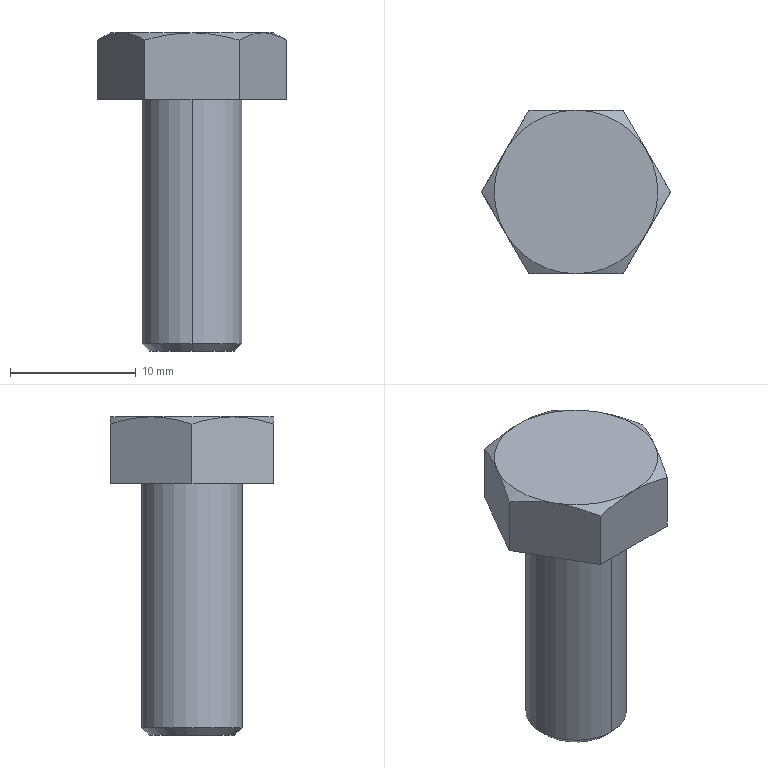Part | SolidWorks | features BaseBody 1 | 1 solid | 19 faces | box 15.011 x 13 x 25.3 mm | volume 1774 mm3 | plane 9 | cone 8 | cylinder 2 | commonest cylinder face diameters 8 x2
STEP:
#1=CARTESIAN_POINT('',(172.5,-20.6,38.));
#2=VERTEX_POINT('',#1);
#3=CARTESIAN_POINT('',(172.5,-27.4,38.));
#4=VERTEX_POINT('',#3);
#5=CARTESIAN_POINT('',(172.5,-24.,38.));
#6=DIRECTION('',(0.,0.,-1.));
#7=DIRECTION('',(0.,1.,0.));
#8=AXIS2_PLACEMENT_3D('',#5,#6,#7);
#9=CIRCLE('',#8,3.4);
#10=EDGE_CURVE('',#2,#4,#9,.T.);
#11=ORIENTED_EDGE('',*,*,#10,.F.);
#12=CARTESIAN_POINT('',(172.5,-20.,38.6));
#13=VERTEX_POINT('',#12);
#14=CARTESIAN_POINT('',(172.5,-20.6,38.));
#15=DIRECTION('',(0.,0.7071,0.7071));
#16=VECTOR('',#15,1000.);
#17=LINE('',#14,#16);
#18=EDGE_CURVE('',#2,#13,#17,.T.);
#19=ORIENTED_EDGE('',*,*,#18,.T.);
#20=CARTESIAN_POINT('',(172.5,-28.,38.6));
#21=VERTEX_POINT('',#20);
#22=CARTESIAN_POINT('',(172.5,-24.,38.6));
#23=DIRECTION('',(0.,0.,1.));
#24=DIRECTION('',(0.,1.,0.));
#25=AXIS2_PLACEMENT_3D('',#22,#23,#24);
#26=CIRCLE('',#25,4.);
#27=EDGE_CURVE('',#21,#13,#26,.T.);
#28=ORIENTED_EDGE('',*,*,#27,.F.);
#29=CARTESIAN_POINT('',(172.5,-27.4,38.));
#30=DIRECTION('',(0.,-0.7071,0.7071));
#31=VECTOR('',#30,1000.);
#32=LINE('',#29,#31);
#33=EDGE_CURVE('',#4,#21,#32,.T.);
#34=ORIENTED_EDGE('',*,*,#33,.F.);
#35=EDGE_LOOP('',(#11,#19,#28,#34));
#36=FACE_OUTER_BOUND('',#35,.T.);
#37=CARTESIAN_POINT('',(172.5,-24.,38.));
#38=DIRECTION('',(0.,0.,1.));
#39=DIRECTION('',(0.,-1.,0.));
#40=AXIS2_PLACEMENT_3D('',#37,#38,#39);
#41=CONICAL_SURFACE('',#40,3.4,0.7854);
#42=ADVANCED_FACE('',(#36),#41,.T.);
#43=ORIENTED_EDGE('',*,*,#27,.T.);
#44=CARTESIAN_POINT('',(172.5,-20.,58.));
#45=VERTEX_POINT('',#44);
#46=CARTESIAN_POINT('',(172.5,-20.,38.));
#47=DIRECTION('',(0.,0.,1.));
#48=VECTOR('',#47,1000.);
#49=LINE('',#46,#48);
#50=EDGE_CURVE('',#13,#45,#49,.T.);
#51=ORIENTED_EDGE('',*,*,#50,.T.);
#52=CARTESIAN_POINT('',(172.5,-28.,58.));
#53=VERTEX_POINT('',#52);
#54=CARTESIAN_POINT('',(172.5,-24.,58.));
#55=DIRECTION('',(0.,0.,-1.));
#56=DIRECTION('',(0.,-1.,0.));
#57=AXIS2_PLACEMENT_3D('',#54,#55,#56);
#58=CIRCLE('',#57,4.);
#59=EDGE_CURVE('',#45,#53,#58,.T.);
#60=ORIENTED_EDGE('',*,*,#59,.T.);
#61=CARTESIAN_POINT('',(172.5,-28.,38.));
#62=DIRECTION('',(0.,0.,1.));
#63=VECTOR('',#62,1000.);
#64=LINE('',#61,#63);
#65=EDGE_CURVE('',#21,#53,#64,.T.);
#66=ORIENTED_EDGE('',*,*,#65,.F.);
#67=EDGE_LOOP('',(#43,#51,#60,#66));
#68=FACE_OUTER_BOUND('',#67,.T.);
#69=CARTESIAN_POINT('',(172.5,-24.,38.));
#70=DIRECTION('',(0.,0.,1.));
#71=DIRECTION('',(0.,-1.,0.));
#72=AXIS2_PLACEMENT_3D('',#69,#70,#71);
#73=CYLINDRICAL_SURFACE('',#72,4.);
#74=ADVANCED_FACE('',(#68),#73,.T.);
#75=CARTESIAN_POINT('',(168.747,-30.5,58.));
#76=VERTEX_POINT('',#75);
#77=CARTESIAN_POINT('',(164.994,-24.,58.));
#78=VERTEX_POINT('',#77);
#79=CARTESIAN_POINT('',(168.747,-30.5,58.));
#80=DIRECTION('',(-0.5,0.866,0.));
#81=VECTOR('',#80,1000.);
#82=LINE('',#79,#81);
#83=EDGE_CURVE('',#76,#78,#82,.T.);
#84=ORIENTED_EDGE('',*,*,#83,.T.);
#85=CARTESIAN_POINT('',(168.747,-17.5,58.));
#86=VERTEX_POINT('',#85);
#87=CARTESIAN_POINT('',(164.994,-24.,58.));
#88=DIRECTION('',(0.5,0.866,0.));
#89=VECTOR('',#88,1000.);
#90=LINE('',#87,#89);
#91=EDGE_CURVE('',#78,#86,#90,.T.);
#92=ORIENTED_EDGE('',*,*,#91,.T.);
#93=CARTESIAN_POINT('',(176.253,-17.5,58.));
#94=VERTEX_POINT('',#93);
#95=CARTESIAN_POINT('',(168.747,-17.5,58.));
#96=DIRECTION('',(1.,0.,0.));
#97=VECTOR('',#96,1000.);
#98=LINE('',#95,#97);
#99=EDGE_CURVE('',#86,#94,#98,.T.);
#100=ORIENTED_EDGE('',*,*,#99,.T.);
#101=CARTESIAN_POINT('',(180.006,-24.,58.));
#102=VERTEX_POINT('',#101);
#103=CARTESIAN_POINT('',(176.253,-17.5,58.));
#104=DIRECTION('',(0.5,-0.866,0.));
#105=VECTOR('',#104,1000.);
#106=LINE('',#103,#105);
#107=EDGE_CURVE('',#94,#102,#106,.T.);
#108=ORIENTED_EDGE('',*,*,#107,.T.);
#109=CARTESIAN_POINT('',(176.253,-30.5,58.));
#110=VERTEX_POINT('',#109);
#111=CARTESIAN_POINT('',(180.006,-24.,58.));
#112=DIRECTION('',(-0.5,-0.866,0.));
#113=VECTOR('',#112,1000.);
#114=LINE('',#111,#113);
#115=EDGE_CURVE('',#102,#110,#114,.T.);
#116=ORIENTED_EDGE('',*,*,#115,.T.);
#117=CARTESIAN_POINT('',(176.253,-30.5,58.));
#118=DIRECTION('',(-1.,0.,0.));
#119=VECTOR('',#118,1000.);
#120=LINE('',#117,#119);
#121=EDGE_CURVE('',#110,#76,#120,.T.);
#122=ORIENTED_EDGE('',*,*,#121,.T.);
#123=EDGE_LOOP('',(#84,#92,#100,#108,#116,#122));
#124=FACE_OUTER_BOUND('',#123,.T.);
#125=CARTESIAN_POINT('',(172.5,-24.,58.));
#126=DIRECTION('',(0.,0.,-1.));
#127=DIRECTION('',(0.,-1.,0.));
#128=AXIS2_PLACEMENT_3D('',#125,#126,#127);
#129=CIRCLE('',#128,4.);
#130=EDGE_CURVE('',#53,#45,#129,.T.);
#131=ORIENTED_EDGE('',*,*,#130,.F.);
#132=ORIENTED_EDGE('',*,*,#59,.F.);
#133=EDGE_LOOP('',(#131,#132));
#134=FACE_BOUND('',#133,.T.);
#135=CARTESIAN_POINT('',(172.5,-37.,58.));
#136=DIRECTION('',(0.,0.,1.));
#137=DIRECTION('',(0.,-1.,0.));
#138=AXIS2_PLACEMENT_3D('',#135,#136,#137);
#139=PLANE('',#138);
#140=ADVANCED_FACE('',(#124,#134),#139,.F.);
#141=CARTESIAN_POINT('',(164.994,-24.,62.719));
#142=VERTEX_POINT('',#141);
#143=CARTESIAN_POINT('',(166.871,-27.25,63.3));
#144=VERTEX_POINT('',#143);
#145=CARTESIAN_POINT('',(164.994,-24.,62.719));
#146=CARTESIAN_POINT('',(165.301,-24.532,62.897));
#147=CARTESIAN_POINT('',(165.611,-25.067,63.043));
#148=CARTESIAN_POINT('',(166.235,-26.149,63.245));
#149=CARTESIAN_POINT('',(166.551,-26.696,63.3));
#150=CARTESIAN_POINT('',(166.871,-27.25,63.3));
#151=B_SPLINE_CURVE_WITH_KNOTS('',3,(#145,#146,#147,#148,#149,#150),.UNSPECIFIED.,.F.,.F.,(4,2,4),(0.000000238,0.001899,0.003797),.UNSPECIFIED.);
#152=EDGE_CURVE('',#142,#144,#151,.T.);
#153=ORIENTED_EDGE('',*,*,#152,.F.);
#154=CARTESIAN_POINT('',(164.994,-24.,58.));
#155=DIRECTION('',(0.,0.,1.));
#156=VECTOR('',#155,1000.);
#157=LINE('',#154,#156);
#158=EDGE_CURVE('',#78,#142,#157,.T.);
#159=ORIENTED_EDGE('',*,*,#158,.F.);
#160=ORIENTED_EDGE('',*,*,#83,.F.);
#161=CARTESIAN_POINT('',(168.747,-30.5,62.719));
#162=VERTEX_POINT('',#161);
#163=CARTESIAN_POINT('',(168.747,-30.5,58.));
#164=DIRECTION('',(0.,0.,1.));
#165=VECTOR('',#164,1000.);
#166=LINE('',#163,#165);
#167=EDGE_CURVE('',#76,#162,#166,.T.);
#168=ORIENTED_EDGE('',*,*,#167,.T.);
#169=CARTESIAN_POINT('',(166.871,-27.25,63.3));
#170=CARTESIAN_POINT('',(167.03,-27.526,63.3));
#171=CARTESIAN_POINT('',(167.19,-27.803,63.286));
#172=CARTESIAN_POINT('',(167.506,-28.351,63.233));
#173=CARTESIAN_POINT('',(167.664,-28.623,63.194));
#174=CARTESIAN_POINT('',(168.132,-29.435,63.042));
#175=CARTESIAN_POINT('',(168.441,-29.97,62.896));
#176=CARTESIAN_POINT('',(168.747,-30.5,62.719));
#177=B_SPLINE_CURVE_WITH_KNOTS('',3,(#169,#170,#171,#172,#173,#174,#175,#176),.UNSPECIFIED.,.F.,.F.,(4,2,2,4),(0.003797,0.004743,0.005689,0.00758),.UNSPECIFIED.);
#178=EDGE_CURVE('',#144,#162,#177,.T.);
#179=ORIENTED_EDGE('',*,*,#178,.F.);
#180=EDGE_LOOP('',(#153,#159,#160,#168,#179));
#181=FACE_OUTER_BOUND('',#180,.T.);
#182=CARTESIAN_POINT('',(168.747,-30.5,58.));
#183=DIRECTION('',(0.866,0.5,0.));
#184=DIRECTION('',(0.5,-0.866,0.));
#185=AXIS2_PLACEMENT_3D('',#182,#183,#184);
#186=PLANE('',#185);
#187=ADVANCED_FACE('',(#181),#186,.F.);
#188=CARTESIAN_POINT('',(168.747,-17.5,62.719));
#189=VERTEX_POINT('',#188);
#190=CARTESIAN_POINT('',(166.871,-20.75,63.3));
#191=VERTEX_POINT('',#190);
#192=CARTESIAN_POINT('',(168.747,-17.5,62.719));
#193=CARTESIAN_POINT('',(168.44,-18.032,62.897));
#194=CARTESIAN_POINT('',(168.131,-18.567,63.043));
#195=CARTESIAN_POINT('',(167.506,-19.649,63.245));
#196=CARTESIAN_POINT('',(167.191,-20.196,63.3));
#197=CARTESIAN_POINT('',(166.871,-20.75,63.3));
#198=B_SPLINE_CURVE_WITH_KNOTS('',3,(#192,#193,#194,#195,#196,#197),.UNSPECIFIED.,.F.,.F.,(4,2,4),(0.000000238,0.001899,0.003797),.UNSPECIFIED.);
#199=EDGE_CURVE('',#189,#191,#198,.T.);
#200=ORIENTED_EDGE('',*,*,#199,.F.);
#201=CARTESIAN_POINT('',(168.747,-17.5,58.));
#202=DIRECTION('',(0.,0.,1.));
#203=VECTOR('',#202,1000.);
#204=LINE('',#201,#203);
#205=EDGE_CURVE('',#86,#189,#204,.T.);
#206=ORIENTED_EDGE('',*,*,#205,.F.);
#207=ORIENTED_EDGE('',*,*,#91,.F.);
#208=ORIENTED_EDGE('',*,*,#158,.T.);
#209=CARTESIAN_POINT('',(166.871,-20.75,63.3));
#210=CARTESIAN_POINT('',(166.712,-21.026,63.3));
#211=CARTESIAN_POINT('',(166.552,-21.303,63.286));
#212=CARTESIAN_POINT('',(166.235,-21.851,63.233));
#213=CARTESIAN_POINT('',(166.078,-22.123,63.194));
#214=CARTESIAN_POINT('',(165.609,-22.935,63.042));
#215=CARTESIAN_POINT('',(165.301,-23.47,62.896));
#216=CARTESIAN_POINT('',(164.994,-24.,62.719));
#217=B_SPLINE_CURVE_WITH_KNOTS('',3,(#209,#210,#211,#212,#213,#214,#215,#216),.UNSPECIFIED.,.F.,.F.,(4,2,2,4),(0.003797,0.004743,0.005689,0.00758),.UNSPECIFIED.);
#218=EDGE_CURVE('',#191,#142,#217,.T.);
#219=ORIENTED_EDGE('',*,*,#218,.F.);
#220=EDGE_LOOP('',(#200,#206,#207,#208,#219));
#221=FACE_OUTER_BOUND('',#220,.T.);
#222=CARTESIAN_POINT('',(164.994,-24.,58.));
#223=DIRECTION('',(0.866,-0.5,0.));
#224=DIRECTION('',(-0.5,-0.866,0.));
#225=AXIS2_PLACEMENT_3D('',#222,#223,#224);
#226=PLANE('',#225);
#227=ADVANCED_FACE('',(#221),#226,.F.);
#228=CARTESIAN_POINT('',(176.253,-17.5,62.719));
#229=VERTEX_POINT('',#228);
#230=CARTESIAN_POINT('',(172.5,-17.5,63.3));
#231=VERTEX_POINT('',#230);
#232=CARTESIAN_POINT('',(176.253,-17.5,62.719));
#233=CARTESIAN_POINT('',(175.646,-17.5,62.895));
#234=CARTESIAN_POINT('',(175.031,-17.5,63.04));
#235=CARTESIAN_POINT('',(173.779,-17.5,63.244));
#236=CARTESIAN_POINT('',(173.136,-17.5,63.3));
#237=CARTESIAN_POINT('',(172.5,-17.5,63.3));
#238=B_SPLINE_CURVE_WITH_KNOTS('',3,(#232,#233,#234,#235,#236,#237),.UNSPECIFIED.,.F.,.F.,(4,2,4),(0.02005,0.02195,0.02385),.UNSPECIFIED.);
#239=EDGE_CURVE('',#229,#231,#238,.T.);
#240=ORIENTED_EDGE('',*,*,#239,.F.);
#241=CARTESIAN_POINT('',(176.253,-17.5,58.));
#242=DIRECTION('',(0.,0.,1.));
#243=VECTOR('',#242,1000.);
#244=LINE('',#241,#243);
#245=EDGE_CURVE('',#94,#229,#244,.T.);
#246=ORIENTED_EDGE('',*,*,#245,.F.);
#247=ORIENTED_EDGE('',*,*,#99,.F.);
#248=ORIENTED_EDGE('',*,*,#205,.T.);
#249=CARTESIAN_POINT('',(172.5,-17.5,63.3));
#250=CARTESIAN_POINT('',(171.865,-17.5,63.3));
#251=CARTESIAN_POINT('',(171.235,-17.5,63.245));
#252=CARTESIAN_POINT('',(169.983,-17.5,63.043));
#253=CARTESIAN_POINT('',(169.358,-17.5,62.896));
#254=CARTESIAN_POINT('',(168.747,-17.5,62.719));
#255=B_SPLINE_CURVE_WITH_KNOTS('',3,(#249,#250,#251,#252,#253,#254),.UNSPECIFIED.,.F.,.F.,(4,2,4),(0.02385,0.02575,0.02765),.UNSPECIFIED.);
#256=EDGE_CURVE('',#231,#189,#255,.T.);
#257=ORIENTED_EDGE('',*,*,#256,.F.);
#258=EDGE_LOOP('',(#240,#246,#247,#248,#257));
#259=FACE_OUTER_BOUND('',#258,.T.);
#260=CARTESIAN_POINT('',(168.747,-17.5,58.));
#261=DIRECTION('',(0.,-1.,0.));
#262=DIRECTION('',(0.,0.,-1.));
#263=AXIS2_PLACEMENT_3D('',#260,#261,#262);
#264=PLANE('',#263);
#265=ADVANCED_FACE('',(#259),#264,.F.);
#266=CARTESIAN_POINT('',(180.006,-24.,62.719));
#267=VERTEX_POINT('',#266);
#268=CARTESIAN_POINT('',(178.129,-20.75,63.3));
#269=VERTEX_POINT('',#268);
#270=CARTESIAN_POINT('',(180.006,-24.,62.719));
#271=CARTESIAN_POINT('',(179.699,-23.468,62.897));
#272=CARTESIAN_POINT('',(179.389,-22.933,63.043));
#273=CARTESIAN_POINT('',(178.765,-21.851,63.245));
#274=CARTESIAN_POINT('',(178.449,-21.304,63.3));
#275=CARTESIAN_POINT('',(178.129,-20.75,63.3));
#276=B_SPLINE_CURVE_WITH_KNOTS('',3,(#270,#271,#272,#273,#274,#275),.UNSPECIFIED.,.F.,.F.,(4,2,4),(0.000000238,0.001899,0.003797),.UNSPECIFIED.);
#277=EDGE_CURVE('',#267,#269,#276,.T.);
#278=ORIENTED_EDGE('',*,*,#277,.F.);
#279=CARTESIAN_POINT('',(180.006,-24.,58.));
#280=DIRECTION('',(0.,0.,1.));
#281=VECTOR('',#280,1000.);
#282=LINE('',#279,#281);
#283=EDGE_CURVE('',#102,#267,#282,.T.);
#284=ORIENTED_EDGE('',*,*,#283,.F.);
#285=ORIENTED_EDGE('',*,*,#107,.F.);
#286=ORIENTED_EDGE('',*,*,#245,.T.);
#287=CARTESIAN_POINT('',(178.129,-20.75,63.3));
#288=CARTESIAN_POINT('',(177.97,-20.474,63.3));
#289=CARTESIAN_POINT('',(177.81,-20.197,63.286));
#290=CARTESIAN_POINT('',(177.494,-19.649,63.233));
#291=CARTESIAN_POINT('',(177.336,-19.377,63.194));
#292=CARTESIAN_POINT('',(176.868,-18.565,63.042));
#293=CARTESIAN_POINT('',(176.559,-18.03,62.896));
#294=CARTESIAN_POINT('',(176.253,-17.5,62.719));
#295=B_SPLINE_CURVE_WITH_KNOTS('',3,(#287,#288,#289,#290,#291,#292,#293,#294),.UNSPECIFIED.,.F.,.F.,(4,2,2,4),(0.003797,0.004743,0.005689,0.00758),.UNSPECIFIED.);
#296=EDGE_CURVE('',#269,#229,#295,.T.);
#297=ORIENTED_EDGE('',*,*,#296,.F.);
#298=EDGE_LOOP('',(#278,#284,#285,#286,#297));
#299=FACE_OUTER_BOUND('',#298,.T.);
#300=CARTESIAN_POINT('',(176.253,-17.5,58.));
#301=DIRECTION('',(-0.866,-0.5,0.));
#302=DIRECTION('',(-0.5,0.866,0.));
#303=AXIS2_PLACEMENT_3D('',#300,#301,#302);
#304=PLANE('',#303);
#305=ADVANCED_FACE('',(#299),#304,.F.);
#306=CARTESIAN_POINT('',(176.253,-30.5,62.719));
#307=VERTEX_POINT('',#306);
#308=CARTESIAN_POINT('',(178.129,-27.25,63.3));
#309=VERTEX_POINT('',#308);
#310=CARTESIAN_POINT('',(176.253,-30.5,62.719));
#311=CARTESIAN_POINT('',(176.56,-29.968,62.897));
#312=CARTESIAN_POINT('',(176.869,-29.433,63.043));
#313=CARTESIAN_POINT('',(177.494,-28.351,63.245));
#314=CARTESIAN_POINT('',(177.809,-27.804,63.3));
#315=CARTESIAN_POINT('',(178.129,-27.25,63.3));
#316=B_SPLINE_CURVE_WITH_KNOTS('',3,(#310,#311,#312,#313,#314,#315),.UNSPECIFIED.,.F.,.F.,(4,2,4),(0.000000238,0.001899,0.003797),.UNSPECIFIED.);
#317=EDGE_CURVE('',#307,#309,#316,.T.);
#318=ORIENTED_EDGE('',*,*,#317,.F.);
#319=CARTESIAN_POINT('',(176.253,-30.5,58.));
#320=DIRECTION('',(0.,0.,1.));
#321=VECTOR('',#320,1000.);
#322=LINE('',#319,#321);
#323=EDGE_CURVE('',#110,#307,#322,.T.);
#324=ORIENTED_EDGE('',*,*,#323,.F.);
#325=ORIENTED_EDGE('',*,*,#115,.F.);
#326=ORIENTED_EDGE('',*,*,#283,.T.);
#327=CARTESIAN_POINT('',(178.129,-27.25,63.3));
#328=CARTESIAN_POINT('',(178.288,-26.974,63.3));
#329=CARTESIAN_POINT('',(178.448,-26.697,63.286));
#330=CARTESIAN_POINT('',(178.765,-26.149,63.233));
#331=CARTESIAN_POINT('',(178.922,-25.877,63.194));
#332=CARTESIAN_POINT('',(179.391,-25.065,63.042));
#333=CARTESIAN_POINT('',(179.699,-24.53,62.896));
#334=CARTESIAN_POINT('',(180.006,-24.,62.719));
#335=B_SPLINE_CURVE_WITH_KNOTS('',3,(#327,#328,#329,#330,#331,#332,#333,#334),.UNSPECIFIED.,.F.,.F.,(4,2,2,4),(0.003797,0.004743,0.005689,0.00758),.UNSPECIFIED.);
#336=EDGE_CURVE('',#309,#267,#335,.T.);
#337=ORIENTED_EDGE('',*,*,#336,.F.);
#338=EDGE_LOOP('',(#318,#324,#325,#326,#337));
#339=FACE_OUTER_BOUND('',#338,.T.);
#340=CARTESIAN_POINT('',(180.006,-24.,58.));
#341=DIRECTION('',(-0.866,0.5,0.));
#342=DIRECTION('',(0.5,0.866,0.));
#343=AXIS2_PLACEMENT_3D('',#340,#341,#342);
#344=PLANE('',#343);
#345=ADVANCED_FACE('',(#339),#344,.F.);
#346=CARTESIAN_POINT('',(172.5,-30.5,63.3));
#347=VERTEX_POINT('',#346);
#348=CARTESIAN_POINT('',(168.747,-30.5,62.719));
#349=CARTESIAN_POINT('',(169.358,-30.5,62.896));
#350=CARTESIAN_POINT('',(169.983,-30.5,63.043));
#351=CARTESIAN_POINT('',(171.235,-30.5,63.245));
#352=CARTESIAN_POINT('',(171.865,-30.5,63.3));
#353=CARTESIAN_POINT('',(172.5,-30.5,63.3));
#354=B_SPLINE_CURVE_WITH_KNOTS('',3,(#348,#349,#350,#351,#352,#353),.UNSPECIFIED.,.F.,.F.,(4,2,4),(0.007008,0.008907,0.01081),.UNSPECIFIED.);
#355=EDGE_CURVE('',#162,#347,#354,.T.);
#356=ORIENTED_EDGE('',*,*,#355,.F.);
#357=ORIENTED_EDGE('',*,*,#167,.F.);
#358=ORIENTED_EDGE('',*,*,#121,.F.);
#359=ORIENTED_EDGE('',*,*,#323,.T.);
#360=CARTESIAN_POINT('',(172.5,-30.5,63.3));
#361=CARTESIAN_POINT('',(173.136,-30.5,63.3));
#362=CARTESIAN_POINT('',(173.779,-30.5,63.244));
#363=CARTESIAN_POINT('',(175.031,-30.5,63.04));
#364=CARTESIAN_POINT('',(175.646,-30.5,62.895));
#365=CARTESIAN_POINT('',(176.253,-30.5,62.719));
#366=B_SPLINE_CURVE_WITH_KNOTS('',3,(#360,#361,#362,#363,#364,#365),.UNSPECIFIED.,.F.,.F.,(4,2,4),(0.01081,0.01271,0.01461),.UNSPECIFIED.);
#367=EDGE_CURVE('',#347,#307,#366,.T.);
#368=ORIENTED_EDGE('',*,*,#367,.F.);
#369=EDGE_LOOP('',(#356,#357,#358,#359,#368));
#370=FACE_OUTER_BOUND('',#369,.T.);
#371=CARTESIAN_POINT('',(176.253,-30.5,58.));
#372=DIRECTION('',(0.,1.,0.));
#373=DIRECTION('',(0.,0.,1.));
#374=AXIS2_PLACEMENT_3D('',#371,#372,#373);
#375=PLANE('',#374);
#376=ADVANCED_FACE('',(#370),#375,.F.);
#377=ORIENTED_EDGE('',*,*,#178,.T.);
#378=ORIENTED_EDGE('',*,*,#355,.T.);
#379=CARTESIAN_POINT('',(172.5,-24.,63.3));
#380=DIRECTION('',(0.,0.,1.));
#381=DIRECTION('',(0.,-1.,0.));
#382=AXIS2_PLACEMENT_3D('',#379,#380,#381);
#383=CIRCLE('',#382,6.5);
#384=EDGE_CURVE('',#144,#347,#383,.T.);
#385=ORIENTED_EDGE('',*,*,#384,.F.);
#386=EDGE_LOOP('',(#377,#378,#385));
#387=FACE_OUTER_BOUND('',#386,.T.);
#388=CARTESIAN_POINT('',(172.5,-24.,63.3));
#389=DIRECTION('',(0.,0.,-1.));
#390=DIRECTION('',(0.,-1.,0.));
#391=AXIS2_PLACEMENT_3D('',#388,#389,#390);
#392=CONICAL_SURFACE('',#391,6.5,1.047);
#393=ADVANCED_FACE('',(#387),#392,.T.);
#394=ORIENTED_EDGE('',*,*,#218,.T.);
#395=ORIENTED_EDGE('',*,*,#152,.T.);
#396=CARTESIAN_POINT('',(172.5,-24.,63.3));
#397=DIRECTION('',(0.,0.,1.));
#398=DIRECTION('',(0.,-1.,0.));
#399=AXIS2_PLACEMENT_3D('',#396,#397,#398);
#400=CIRCLE('',#399,6.5);
#401=EDGE_CURVE('',#191,#144,#400,.T.);
#402=ORIENTED_EDGE('',*,*,#401,.F.);
#403=EDGE_LOOP('',(#394,#395,#402));
#404=FACE_OUTER_BOUND('',#403,.T.);
#405=CARTESIAN_POINT('',(172.5,-24.,63.3));
#406=DIRECTION('',(0.,0.,-1.));
#407=DIRECTION('',(0.,-1.,0.));
#408=AXIS2_PLACEMENT_3D('',#405,#406,#407);
#409=CONICAL_SURFACE('',#408,6.5,1.047);
#410=ADVANCED_FACE('',(#404),#409,.T.);
#411=ORIENTED_EDGE('',*,*,#256,.T.);
#412=ORIENTED_EDGE('',*,*,#199,.T.);
#413=CARTESIAN_POINT('',(172.5,-24.,63.3));
#414=DIRECTION('',(0.,0.,1.));
#415=DIRECTION('',(0.,-1.,0.));
#416=AXIS2_PLACEMENT_3D('',#413,#414,#415);
#417=CIRCLE('',#416,6.5);
#418=EDGE_CURVE('',#231,#191,#417,.T.);
#419=ORIENTED_EDGE('',*,*,#418,.F.);
#420=EDGE_LOOP('',(#411,#412,#419));
#421=FACE_OUTER_BOUND('',#420,.T.);
#422=CARTESIAN_POINT('',(172.5,-24.,63.3));
#423=DIRECTION('',(0.,0.,-1.));
#424=DIRECTION('',(0.,-1.,0.));
#425=AXIS2_PLACEMENT_3D('',#422,#423,#424);
#426=CONICAL_SURFACE('',#425,6.5,1.047);
#427=ADVANCED_FACE('',(#421),#426,.T.);
#428=ORIENTED_EDGE('',*,*,#239,.T.);
#429=CARTESIAN_POINT('',(172.5,-24.,63.3));
#430=DIRECTION('',(0.,0.,1.));
#431=DIRECTION('',(0.,-1.,0.));
#432=AXIS2_PLACEMENT_3D('',#429,#430,#431);
#433=CIRCLE('',#432,6.5);
#434=EDGE_CURVE('',#269,#231,#433,.T.);
#435=ORIENTED_EDGE('',*,*,#434,.F.);
#436=ORIENTED_EDGE('',*,*,#296,.T.);
#437=EDGE_LOOP('',(#428,#435,#436));
#438=FACE_OUTER_BOUND('',#437,.T.);
#439=CARTESIAN_POINT('',(172.5,-24.,63.3));
#440=DIRECTION('',(0.,0.,-1.));
#441=DIRECTION('',(0.,-1.,0.));
#442=AXIS2_PLACEMENT_3D('',#439,#440,#441);
#443=CONICAL_SURFACE('',#442,6.5,1.047);
#444=ADVANCED_FACE('',(#438),#443,.T.);
#445=ORIENTED_EDGE('',*,*,#277,.T.);
#446=CARTESIAN_POINT('',(172.5,-24.,63.3));
#447=DIRECTION('',(0.,0.,1.));
#448=DIRECTION('',(0.,-1.,0.));
#449=AXIS2_PLACEMENT_3D('',#446,#447,#448);
#450=CIRCLE('',#449,6.5);
#451=EDGE_CURVE('',#309,#269,#450,.T.);
#452=ORIENTED_EDGE('',*,*,#451,.F.);
#453=ORIENTED_EDGE('',*,*,#336,.T.);
#454=EDGE_LOOP('',(#445,#452,#453));
#455=FACE_OUTER_BOUND('',#454,.T.);
#456=CARTESIAN_POINT('',(172.5,-24.,63.3));
#457=DIRECTION('',(0.,0.,-1.));
#458=DIRECTION('',(0.,-1.,0.));
#459=AXIS2_PLACEMENT_3D('',#456,#457,#458);
#460=CONICAL_SURFACE('',#459,6.5,1.047);
#461=ADVANCED_FACE('',(#455),#460,.T.);
#462=ORIENTED_EDGE('',*,*,#317,.T.);
#463=CARTESIAN_POINT('',(172.5,-24.,63.3));
#464=DIRECTION('',(0.,0.,1.));
#465=DIRECTION('',(0.,-1.,0.));
#466=AXIS2_PLACEMENT_3D('',#463,#464,#465);
#467=CIRCLE('',#466,6.5);
#468=EDGE_CURVE('',#347,#309,#467,.T.);
#469=ORIENTED_EDGE('',*,*,#468,.F.);
#470=ORIENTED_EDGE('',*,*,#367,.T.);
#471=EDGE_LOOP('',(#462,#469,#470));
#472=FACE_OUTER_BOUND('',#471,.T.);
#473=CARTESIAN_POINT('',(172.5,-24.,63.3));
#474=DIRECTION('',(0.,0.,-1.));
#475=DIRECTION('',(0.,-1.,0.));
#476=AXIS2_PLACEMENT_3D('',#473,#474,#475);
#477=CONICAL_SURFACE('',#476,6.5,1.047);
#478=ADVANCED_FACE('',(#472),#477,.T.);
#479=ORIENTED_EDGE('',*,*,#384,.T.);
#480=ORIENTED_EDGE('',*,*,#468,.T.);
#481=ORIENTED_EDGE('',*,*,#451,.T.);
#482=ORIENTED_EDGE('',*,*,#434,.T.);
#483=ORIENTED_EDGE('',*,*,#418,.T.);
#484=ORIENTED_EDGE('',*,*,#401,.T.);
#485=EDGE_LOOP('',(#479,#480,#481,#482,#483,#484));
#486=FACE_OUTER_BOUND('',#485,.T.);
#487=CARTESIAN_POINT('',(172.5,-37.,63.3));
#488=DIRECTION('',(0.,0.,1.));
#489=DIRECTION('',(0.,-1.,0.));
#490=AXIS2_PLACEMENT_3D('',#487,#488,#489);
#491=PLANE('',#490);
#492=ADVANCED_FACE('',(#486),#491,.T.);
#493=ORIENTED_EDGE('',*,*,#50,.F.);
#494=CARTESIAN_POINT('',(172.5,-24.,38.6));
#495=DIRECTION('',(0.,0.,1.));
#496=DIRECTION('',(0.,1.,0.));
#497=AXIS2_PLACEMENT_3D('',#494,#495,#496);
#498=CIRCLE('',#497,4.);
#499=EDGE_CURVE('',#13,#21,#498,.T.);
#500=ORIENTED_EDGE('',*,*,#499,.T.);
#501=ORIENTED_EDGE('',*,*,#65,.T.);
#502=ORIENTED_EDGE('',*,*,#130,.T.);
#503=EDGE_LOOP('',(#493,#500,#501,#502));
#504=FACE_OUTER_BOUND('',#503,.T.);
#505=CARTESIAN_POINT('',(172.5,-24.,38.));
#506=DIRECTION('',(0.,0.,1.));
#507=DIRECTION('',(0.,-1.,0.));
#508=AXIS2_PLACEMENT_3D('',#505,#506,#507);
#509=CYLINDRICAL_SURFACE('',#508,4.);
#510=ADVANCED_FACE('',(#504),#509,.T.);
#511=CARTESIAN_POINT('',(172.5,-24.,38.));
#512=DIRECTION('',(0.,0.,-1.));
#513=DIRECTION('',(0.,1.,0.));
#514=AXIS2_PLACEMENT_3D('',#511,#512,#513);
#515=CIRCLE('',#514,3.4);
#516=EDGE_CURVE('',#4,#2,#515,.T.);
#517=ORIENTED_EDGE('',*,*,#516,.T.);
#518=ORIENTED_EDGE('',*,*,#10,.T.);
#519=EDGE_LOOP('',(#517,#518));
#520=FACE_OUTER_BOUND('',#519,.T.);
#521=CARTESIAN_POINT('',(172.5,-24.,38.));
#522=DIRECTION('',(0.,0.,-1.));
#523=DIRECTION('',(0.,1.,0.));
#524=AXIS2_PLACEMENT_3D('',#521,#522,#523);
#525=PLANE('',#524);
#526=ADVANCED_FACE('',(#520),#525,.T.);
#527=ORIENTED_EDGE('',*,*,#18,.F.);
#528=ORIENTED_EDGE('',*,*,#516,.F.);
#529=ORIENTED_EDGE('',*,*,#33,.T.);
#530=ORIENTED_EDGE('',*,*,#499,.F.);
#531=EDGE_LOOP('',(#527,#528,#529,#530));
#532=FACE_OUTER_BOUND('',#531,.T.);
#533=CARTESIAN_POINT('',(172.5,-24.,38.));
#534=DIRECTION('',(0.,0.,1.));
#535=DIRECTION('',(0.,-1.,0.));
#536=AXIS2_PLACEMENT_3D('',#533,#534,#535);
#537=CONICAL_SURFACE('',#536,3.4,0.7854);
#538=ADVANCED_FACE('',(#532),#537,.T.);
#539=CLOSED_SHELL('',(#42,#74,#140,#187,#227,#265,#305,#345,#376,#393,#410,#427,#444,#461,#478,#492,#510,#526,#538));
#540=MANIFOLD_SOLID_BREP('',#539);
#541=CARTESIAN_POINT('',(0.,0.,0.));
#542=DIRECTION('',(0.,0.,1.));
#543=DIRECTION('',(1.,0.,0.));
#544=AXIS2_PLACEMENT_3D('',#541,#542,#543);
#545=(LENGTH_UNIT()NAMED_UNIT(*)SI_UNIT(.MILLI.,.METRE.));
#546=UNCERTAINTY_MEASURE_WITH_UNIT(LENGTH_MEASURE(0.00001),#545,'','');
#547=(NAMED_UNIT(*)PLANE_ANGLE_UNIT()SI_UNIT($,.RADIAN.));
#548=(NAMED_UNIT(*)SI_UNIT($,.STERADIAN.)SOLID_ANGLE_UNIT());
#549=(GEOMETRIC_REPRESENTATION_CONTEXT(3)GLOBAL_UNCERTAINTY_ASSIGNED_CONTEXT((#546))GLOBAL_UNIT_ASSIGNED_CONTEXT((#545,#547,#548))REPRESENTATION_CONTEXT('',''));
#550=ADVANCED_BREP_SHAPE_REPRESENTATION('',(#540,#544),#549);